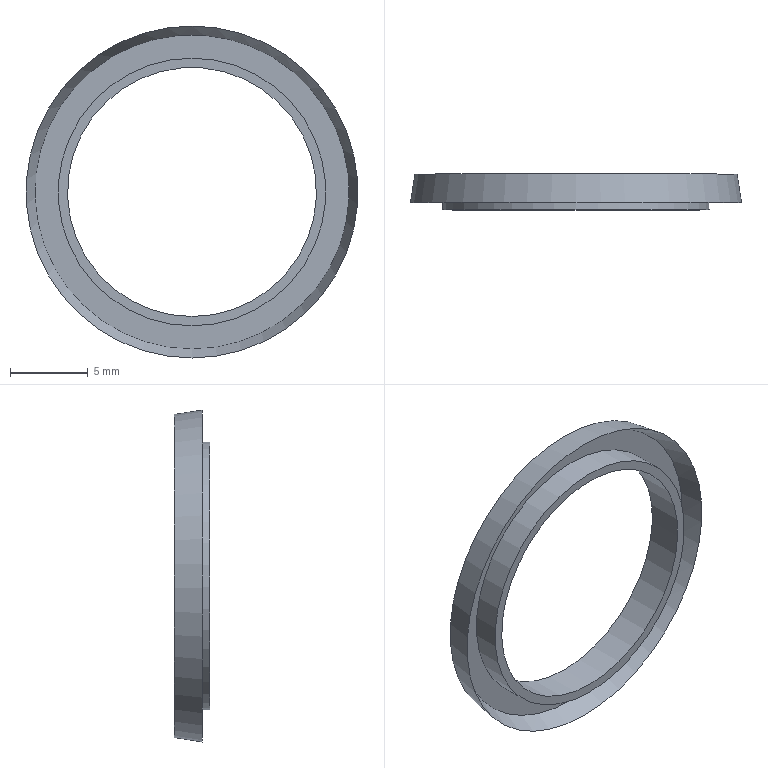Part | NX | features DATUM_CSYS 3, SKETCH 2, SWP104 1 | 1 solid | 7 faces | box 21.341 x 2.3 x 21.341 mm | volume 152.879 mm3 | plane 3 | cone 2 | cylinder 2 | commonest cylinder face diameters 16 x1 17.2 x1
STEP:
#1=CARTESIAN_POINT('',(0.,0.,-10.1));
#2=VERTEX_POINT('',#1);
#3=CARTESIAN_POINT('',(0.,0.,0.));
#4=DIRECTION('',(0.,-1.,0.));
#5=DIRECTION('',(0.,0.,-1.));
#6=AXIS2_PLACEMENT_3D('',#3,#4,#5);
#7=CIRCLE('',#6,10.1);
#8=EDGE_CURVE('',#2,#2,#7,.T.);
#9=ORIENTED_EDGE('',*,*,#8,.T.);
#10=EDGE_LOOP('',(#9));
#11=FACE_BOUND('',#10,.T.);
#12=CARTESIAN_POINT('',(0.,0.,-8.6));
#13=VERTEX_POINT('',#12);
#14=CARTESIAN_POINT('',(0.,0.,0.));
#15=DIRECTION('',(0.,-1.,0.));
#16=DIRECTION('',(0.,0.,-1.));
#17=AXIS2_PLACEMENT_3D('',#14,#15,#16);
#18=CIRCLE('',#17,8.6);
#19=EDGE_CURVE('',#13,#13,#18,.T.);
#20=ORIENTED_EDGE('',*,*,#19,.F.);
#21=EDGE_LOOP('',(#20));
#22=FACE_BOUND('',#21,.T.);
#23=CARTESIAN_POINT('',(0.,0.,8.6));
#24=DIRECTION('',(0.,-1.,0.));
#25=DIRECTION('',(0.,0.,-1.));
#26=AXIS2_PLACEMENT_3D('',#23,#24,#25);
#27=PLANE('',#26);
#28=ADVANCED_FACE('',(#11,#22),#27,.T.);
#29=CARTESIAN_POINT('',(0.,-1.224,-10.671));
#30=VERTEX_POINT('',#29);
#31=CARTESIAN_POINT('',(0.,-1.224,0.));
#32=DIRECTION('',(0.,-1.,0.));
#33=DIRECTION('',(0.,0.,-1.));
#34=AXIS2_PLACEMENT_3D('',#31,#32,#33);
#35=CIRCLE('',#34,10.671);
#36=EDGE_CURVE('',#30,#30,#35,.T.);
#37=ORIENTED_EDGE('',*,*,#36,.T.);
#38=EDGE_LOOP('',(#37));
#39=FACE_BOUND('',#38,.T.);
#40=ORIENTED_EDGE('',*,*,#8,.F.);
#41=EDGE_LOOP('',(#40));
#42=FACE_BOUND('',#41,.T.);
#43=CARTESIAN_POINT('',(0.,0.,0.));
#44=DIRECTION('',(0.,-1.,0.));
#45=DIRECTION('',(0.,0.,-1.));
#46=AXIS2_PLACEMENT_3D('',#43,#44,#45);
#47=CONICAL_SURFACE('',#46,10.1,0.4363);
#48=ADVANCED_FACE('',(#39,#42),#47,.F.);
#49=CARTESIAN_POINT('',(0.,0.6,-10.385));
#50=VERTEX_POINT('',#49);
#51=CARTESIAN_POINT('',(0.,0.6,0.));
#52=DIRECTION('',(0.,-1.,0.));
#53=DIRECTION('',(0.,0.,-1.));
#54=AXIS2_PLACEMENT_3D('',#51,#52,#53);
#55=CIRCLE('',#54,10.385);
#56=EDGE_CURVE('',#50,#50,#55,.T.);
#57=ORIENTED_EDGE('',*,*,#56,.T.);
#58=EDGE_LOOP('',(#57));
#59=FACE_BOUND('',#58,.T.);
#60=ORIENTED_EDGE('',*,*,#36,.F.);
#61=EDGE_LOOP('',(#60));
#62=FACE_BOUND('',#61,.T.);
#63=CARTESIAN_POINT('',(0.,-1.224,0.));
#64=DIRECTION('',(0.,-1.,0.));
#65=DIRECTION('',(0.,0.,-1.));
#66=AXIS2_PLACEMENT_3D('',#63,#64,#65);
#67=CONICAL_SURFACE('',#66,10.671,0.1552);
#68=ADVANCED_FACE('',(#59,#62),#67,.T.);
#69=CARTESIAN_POINT('',(0.,0.6,-8.));
#70=VERTEX_POINT('',#69);
#71=CARTESIAN_POINT('',(0.,0.6,0.));
#72=DIRECTION('',(0.,-1.,0.));
#73=DIRECTION('',(0.,0.,-1.));
#74=AXIS2_PLACEMENT_3D('',#71,#72,#73);
#75=CIRCLE('',#74,8.);
#76=EDGE_CURVE('',#70,#70,#75,.T.);
#77=ORIENTED_EDGE('',*,*,#76,.T.);
#78=EDGE_LOOP('',(#77));
#79=FACE_BOUND('',#78,.T.);
#80=ORIENTED_EDGE('',*,*,#56,.F.);
#81=EDGE_LOOP('',(#80));
#82=FACE_BOUND('',#81,.T.);
#83=CARTESIAN_POINT('',(0.,0.6,10.1));
#84=DIRECTION('',(0.,1.,0.));
#85=DIRECTION('',(0.,0.,1.));
#86=AXIS2_PLACEMENT_3D('',#83,#84,#85);
#87=PLANE('',#86);
#88=ADVANCED_FACE('',(#79,#82),#87,.T.);
#89=CARTESIAN_POINT('',(0.,-1.7,-8.));
#90=VERTEX_POINT('',#89);
#91=CARTESIAN_POINT('',(0.,-1.7,0.));
#92=DIRECTION('',(0.,-1.,0.));
#93=DIRECTION('',(0.,0.,-1.));
#94=AXIS2_PLACEMENT_3D('',#91,#92,#93);
#95=CIRCLE('',#94,8.);
#96=EDGE_CURVE('',#90,#90,#95,.T.);
#97=ORIENTED_EDGE('',*,*,#96,.T.);
#98=EDGE_LOOP('',(#97));
#99=FACE_BOUND('',#98,.T.);
#100=ORIENTED_EDGE('',*,*,#76,.F.);
#101=EDGE_LOOP('',(#100));
#102=FACE_BOUND('',#101,.T.);
#103=CARTESIAN_POINT('',(0.,0.,0.));
#104=DIRECTION('',(0.,-1.,0.));
#105=DIRECTION('',(0.,0.,-1.));
#106=AXIS2_PLACEMENT_3D('',#103,#104,#105);
#107=CYLINDRICAL_SURFACE('',#106,8.);
#108=ADVANCED_FACE('',(#99,#102),#107,.F.);
#109=CARTESIAN_POINT('',(0.,-1.7,-8.6));
#110=VERTEX_POINT('',#109);
#111=CARTESIAN_POINT('',(0.,-1.7,0.));
#112=DIRECTION('',(0.,-1.,0.));
#113=DIRECTION('',(0.,0.,-1.));
#114=AXIS2_PLACEMENT_3D('',#111,#112,#113);
#115=CIRCLE('',#114,8.6);
#116=EDGE_CURVE('',#110,#110,#115,.T.);
#117=ORIENTED_EDGE('',*,*,#116,.T.);
#118=EDGE_LOOP('',(#117));
#119=FACE_BOUND('',#118,.T.);
#120=ORIENTED_EDGE('',*,*,#96,.F.);
#121=EDGE_LOOP('',(#120));
#122=FACE_BOUND('',#121,.T.);
#123=CARTESIAN_POINT('',(0.,-1.7,8.));
#124=DIRECTION('',(0.,-1.,0.));
#125=DIRECTION('',(0.,0.,-1.));
#126=AXIS2_PLACEMENT_3D('',#123,#124,#125);
#127=PLANE('',#126);
#128=ADVANCED_FACE('',(#119,#122),#127,.T.);
#129=ORIENTED_EDGE('',*,*,#19,.T.);
#130=EDGE_LOOP('',(#129));
#131=FACE_BOUND('',#130,.T.);
#132=ORIENTED_EDGE('',*,*,#116,.F.);
#133=EDGE_LOOP('',(#132));
#134=FACE_BOUND('',#133,.T.);
#135=CARTESIAN_POINT('',(0.,0.,0.));
#136=DIRECTION('',(0.,-1.,0.));
#137=DIRECTION('',(0.,0.,-1.));
#138=AXIS2_PLACEMENT_3D('',#135,#136,#137);
#139=CYLINDRICAL_SURFACE('',#138,8.6);
#140=ADVANCED_FACE('',(#131,#134),#139,.T.);
#141=CLOSED_SHELL('',(#28,#48,#68,#88,#108,#128,#140));
#142=MANIFOLD_SOLID_BREP('',#141);
#143=(LENGTH_UNIT()NAMED_UNIT(*)SI_UNIT(.MILLI.,.METRE.));
#144=UNCERTAINTY_MEASURE_WITH_UNIT(LENGTH_MEASURE(0.00001),#143,'','');
#145=(NAMED_UNIT(*)PLANE_ANGLE_UNIT()SI_UNIT($,.RADIAN.));
#146=(NAMED_UNIT(*)SI_UNIT($,.STERADIAN.)SOLID_ANGLE_UNIT());
#147=(GEOMETRIC_REPRESENTATION_CONTEXT(3)GLOBAL_UNCERTAINTY_ASSIGNED_CONTEXT((#144))GLOBAL_UNIT_ASSIGNED_CONTEXT((#143,#145,#146))REPRESENTATION_CONTEXT('',''));
#148=ADVANCED_BREP_SHAPE_REPRESENTATION('',(#142),#147);